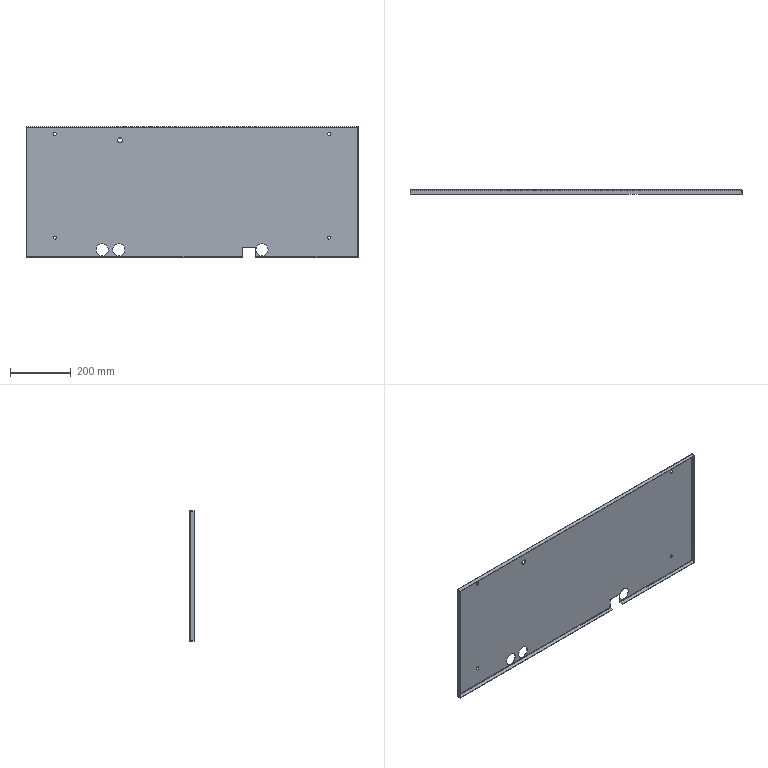Part | 1 solid | 69 faces | box 1090 x 15 x 429.998 mm | volume 752061 mm3 | plane 36 | cylinder 26 | spline 7 | commonest cylinder face diameters 10 x8 40 x6 1.48 x3 4.48 x3 1.473 x2 4.473 x2